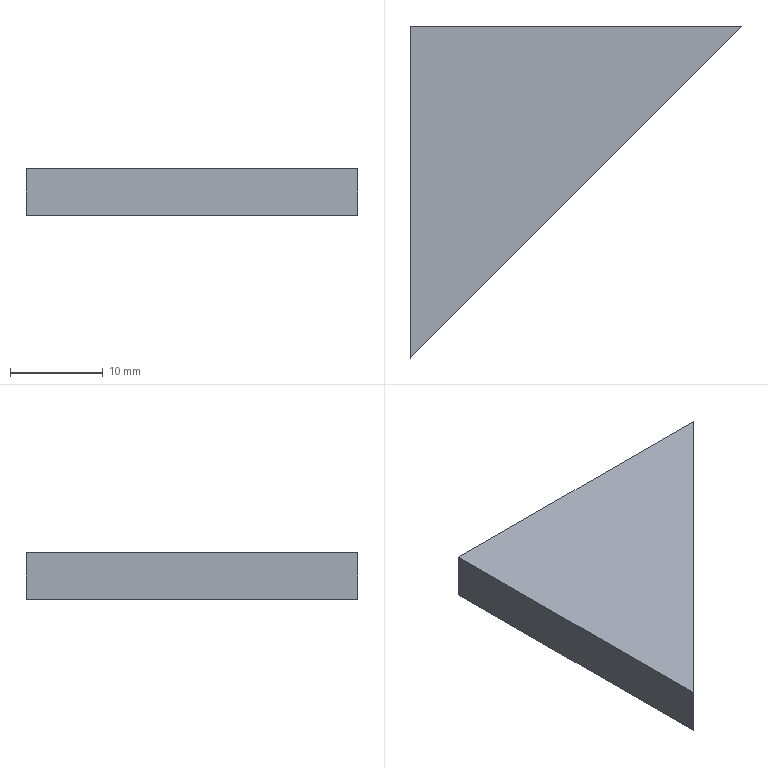Part | NX | features solid 2 | 1 solid | 5 faces | box 35.858 x 35.858 x 5 mm | volume 3214 mm3 | plane 5
STEP:
#1=CARTESIAN_POINT('',(15.,-647.5,-10.));
#2=VERTEX_POINT('',#1);
#3=CARTESIAN_POINT('',(15.,-683.358,-10.));
#4=VERTEX_POINT('',#3);
#5=CARTESIAN_POINT('',(15.,-647.5,-10.));
#6=DIRECTION('',(0.,-1.,0.));
#7=VECTOR('',#6,1000.);
#8=LINE('',#5,#7);
#9=EDGE_CURVE('',#2,#4,#8,.T.);
#10=ORIENTED_EDGE('',*,*,#9,.T.);
#11=CARTESIAN_POINT('',(50.858,-647.5,-10.));
#12=VERTEX_POINT('',#11);
#13=CARTESIAN_POINT('',(57.929,-640.429,-10.));
#14=DIRECTION('',(-0.7071,-0.7071,0.));
#15=VECTOR('',#14,1000.);
#16=LINE('',#13,#15);
#17=EDGE_CURVE('',#4,#12,#16,.F.);
#18=ORIENTED_EDGE('',*,*,#17,.T.);
#19=CARTESIAN_POINT('',(65.,-647.5,-10.));
#20=DIRECTION('',(-1.,0.,0.));
#21=VECTOR('',#20,1000.);
#22=LINE('',#19,#21);
#23=EDGE_CURVE('',#12,#2,#22,.T.);
#24=ORIENTED_EDGE('',*,*,#23,.T.);
#25=EDGE_LOOP('',(#10,#18,#24));
#26=FACE_BOUND('',#25,.T.);
#27=CARTESIAN_POINT('',(65.,-647.5,-10.));
#28=DIRECTION('',(0.,0.,1.));
#29=DIRECTION('',(-1.,0.,0.));
#30=AXIS2_PLACEMENT_3D('',#27,#28,#29);
#31=PLANE('',#30);
#32=ADVANCED_FACE('',(#26),#31,.T.);
#33=ORIENTED_EDGE('',*,*,#9,.F.);
#34=CARTESIAN_POINT('',(15.,-647.5,-15.));
#35=VERTEX_POINT('',#34);
#36=CARTESIAN_POINT('',(15.,-647.5,-20.));
#37=DIRECTION('',(0.,0.,1.));
#38=VECTOR('',#37,1000.);
#39=LINE('',#36,#38);
#40=EDGE_CURVE('',#35,#2,#39,.T.);
#41=ORIENTED_EDGE('',*,*,#40,.F.);
#42=CARTESIAN_POINT('',(15.,-683.358,-15.));
#43=VERTEX_POINT('',#42);
#44=CARTESIAN_POINT('',(15.,-647.5,-15.));
#45=DIRECTION('',(0.,-1.,0.));
#46=VECTOR('',#45,1000.);
#47=LINE('',#44,#46);
#48=EDGE_CURVE('',#35,#43,#47,.T.);
#49=ORIENTED_EDGE('',*,*,#48,.T.);
#50=CARTESIAN_POINT('',(15.,-683.358,-20.));
#51=DIRECTION('',(0.,0.,1.));
#52=VECTOR('',#51,1000.);
#53=LINE('',#50,#52);
#54=EDGE_CURVE('',#43,#4,#53,.T.);
#55=ORIENTED_EDGE('',*,*,#54,.T.);
#56=EDGE_LOOP('',(#33,#41,#49,#55));
#57=FACE_BOUND('',#56,.T.);
#58=CARTESIAN_POINT('',(15.,-647.5,-20.));
#59=DIRECTION('',(1.,0.,0.));
#60=DIRECTION('',(0.,0.,1.));
#61=AXIS2_PLACEMENT_3D('',#58,#59,#60);
#62=PLANE('',#61);
#63=ADVANCED_FACE('',(#57),#62,.F.);
#64=CARTESIAN_POINT('',(50.858,-647.5,-15.));
#65=VERTEX_POINT('',#64);
#66=CARTESIAN_POINT('',(65.,-647.5,-15.));
#67=DIRECTION('',(1.,0.,0.));
#68=VECTOR('',#67,1000.);
#69=LINE('',#66,#68);
#70=EDGE_CURVE('',#65,#35,#69,.F.);
#71=ORIENTED_EDGE('',*,*,#70,.F.);
#72=CARTESIAN_POINT('',(57.929,-640.429,-15.));
#73=DIRECTION('',(-0.7071,-0.7071,0.));
#74=VECTOR('',#73,1000.);
#75=LINE('',#72,#74);
#76=EDGE_CURVE('',#65,#43,#75,.T.);
#77=ORIENTED_EDGE('',*,*,#76,.T.);
#78=ORIENTED_EDGE('',*,*,#48,.F.);
#79=EDGE_LOOP('',(#71,#77,#78));
#80=FACE_BOUND('',#79,.T.);
#81=CARTESIAN_POINT('',(65.,-647.5,-15.));
#82=DIRECTION('',(0.,0.,1.));
#83=DIRECTION('',(-1.,0.,0.));
#84=AXIS2_PLACEMENT_3D('',#81,#82,#83);
#85=PLANE('',#84);
#86=ADVANCED_FACE('',(#80),#85,.F.);
#87=ORIENTED_EDGE('',*,*,#40,.T.);
#88=ORIENTED_EDGE('',*,*,#23,.F.);
#89=CARTESIAN_POINT('',(50.858,-647.5,-20.));
#90=DIRECTION('',(0.,0.,-1.));
#91=VECTOR('',#90,1000.);
#92=LINE('',#89,#91);
#93=EDGE_CURVE('',#65,#12,#92,.F.);
#94=ORIENTED_EDGE('',*,*,#93,.F.);
#95=ORIENTED_EDGE('',*,*,#70,.T.);
#96=EDGE_LOOP('',(#87,#88,#94,#95));
#97=FACE_BOUND('',#96,.T.);
#98=CARTESIAN_POINT('',(65.,-647.5,-20.));
#99=DIRECTION('',(0.,-1.,0.));
#100=DIRECTION('',(0.,0.,1.));
#101=AXIS2_PLACEMENT_3D('',#98,#99,#100);
#102=PLANE('',#101);
#103=ADVANCED_FACE('',(#97),#102,.F.);
#104=ORIENTED_EDGE('',*,*,#76,.F.);
#105=ORIENTED_EDGE('',*,*,#93,.T.);
#106=ORIENTED_EDGE('',*,*,#17,.F.);
#107=ORIENTED_EDGE('',*,*,#54,.F.);
#108=EDGE_LOOP('',(#104,#105,#106,#107));
#109=FACE_BOUND('',#108,.T.);
#110=CARTESIAN_POINT('',(7.929,-690.429,-20.));
#111=DIRECTION('',(-0.7071,0.7071,0.));
#112=DIRECTION('',(-0.7071,-0.7071,0.));
#113=AXIS2_PLACEMENT_3D('',#110,#111,#112);
#114=PLANE('',#113);
#115=ADVANCED_FACE('',(#109),#114,.F.);
#116=CLOSED_SHELL('',(#32,#63,#86,#103,#115));
#117=MANIFOLD_SOLID_BREP('',#116);
#118=(LENGTH_UNIT()NAMED_UNIT(*)SI_UNIT(.MILLI.,.METRE.));
#119=UNCERTAINTY_MEASURE_WITH_UNIT(LENGTH_MEASURE(0.00001),#118,'','');
#120=(NAMED_UNIT(*)PLANE_ANGLE_UNIT()SI_UNIT($,.RADIAN.));
#121=(NAMED_UNIT(*)SI_UNIT($,.STERADIAN.)SOLID_ANGLE_UNIT());
#122=(GEOMETRIC_REPRESENTATION_CONTEXT(3)GLOBAL_UNCERTAINTY_ASSIGNED_CONTEXT((#119))GLOBAL_UNIT_ASSIGNED_CONTEXT((#118,#120,#121))REPRESENTATION_CONTEXT('',''));
#123=ADVANCED_BREP_SHAPE_REPRESENTATION('',(#117),#122);